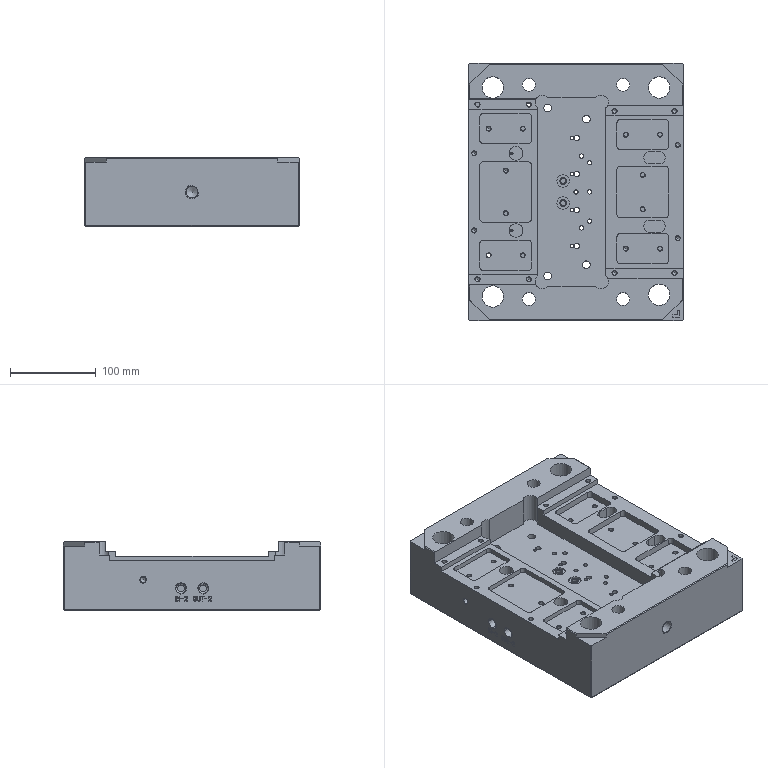NC program | PowerMill | posted with a generic post | part box 250 x 300 x 80 mm
Whole program:
%
O0001
N104 ( POWERMILL CB  : 2026004.0)
N105 ( POST VER      : 2026.0.0.5161)
N106 ( OPTION FILE   : FANUC)
N107 ( OUTPUT WORKPLANE : 2)
N108 (  )
N109 ( TOOL LIST )
N110 (-----------------------------------)
N111 ( NO. | ID    | DIA.| TIP RAD|LENGTH)
N112 (-----------------------------------)
N113 (    1|￠6_2_1| 6.0 |  0.0   |110.36)
N114 (-----------------------------------)
N115 (  )
N116 ( NUMBER OF TOOLPATHS: 1.0 )
N117 ( ESTIMATED PROGRAM DURATION: 0 HOURS 0 MIN 46 SEC)
N118 (  )
N119 G00 G21 G80 G40 G17
N120 G90
N121 G54
N122 G53 Z0.0
N123 (---------------)
N124 ( START TOOLPATH : 25开粗-￠6-钻孔加工 )
N125 (---------------)
N126 ( TOOL NO.    :1 )
N127 ( TOOL TYPE   : DRILL)
N128 ( TOOL ID     : ￠6_2_1)
N129 ( TOOL DIA    : 6.0 LENGTH 110.36)
N130 T1
N131 M6
N132 S700 M03
N133 G00 G90 X13.0 Y15.0
N134 G43 Z20.0 H1
N135
N136 G05 P0
N137 Z-28.5
N138 G01 Z-36.5 F80.0
N139 G00 Z-28.5
N140 Z-35.9
N141 G01 Z-39.5
N142 G00 Z-28.5
N143 Z-38.9
N144 G01 Z-42.5
N145 G00 Z-28.5
N146 Z-41.9
N147 G01 Z-45.5
N148 G00 Z-28.5
N149 Z-44.9
N150 G01 Z-48.5
N151 G00 Z-28.5
N152 Z-47.9
N153 G01 Z-51.5
N154 G00 Z-28.5
N155 Z-50.9
N156 G01 Z-53.5863
N157 G00 Z20.0
N158 X-13.0
N159 Z-28.5
N160 G01 Z-36.5
N161 G00 Z-28.5
N162 Z-35.9
N163 G01 Z-39.5
N164 G00 Z-28.5
N165 Z-38.9
N166 G01 Z-42.5
N167 G00 Z-28.5
N168 Z-41.9
N169 G01 Z-45.5
N170 G00 Z-28.5
N171 Z-44.9
N172 G01 Z-48.5
N173 G00 Z-28.5
N174 Z-47.9
N175 G01 Z-51.5
N176 G00 Z-28.5
N177 Z-50.9
N178 G01 Z-53.5863
N179 G00 Z20.0
N180 G05 P0
N181 (---------------)
N182 ( END TOOLPATH : 25开粗-￠6-钻孔加工 )
N183 (---------------)
N184
N185 M05
N186 G53 Z0.0
N187 M30
%